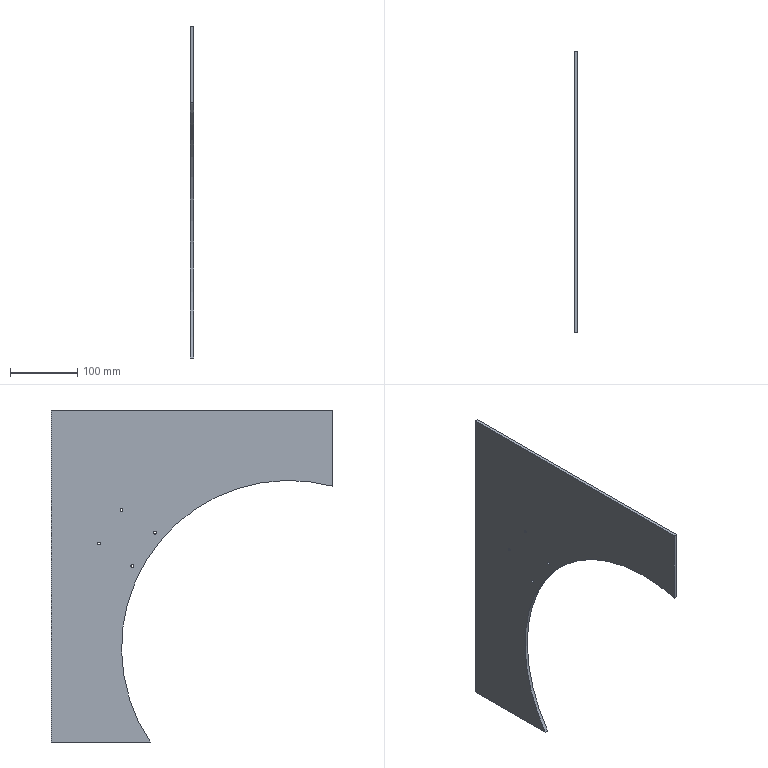Part | STEP file | 09-12 Outer base plate 1 | 1 solid | 15 faces | box 5 x 420 x 495 mm | volume 502595 mm3 | cylinder 9 | plane 6 | commonest cylinder face diameters 4.2 x8 500 x1
STEP:
#1=CARTESIAN_POINT('',(0.,0.,0.));
#2=DIRECTION('',(0.,0.,1.));
#3=DIRECTION('',(1.,0.,0.));
#4=AXIS2_PLACEMENT_3D('',#1,#2,#3);
#5=CARTESIAN_POINT('',(0.,348.664,-201.105));
#6=VERTEX_POINT('',#5);
#7=CARTESIAN_POINT('',(5.,348.664,-201.105));
#8=VERTEX_POINT('',#7);
#9=CARTESIAN_POINT('',(0.,348.664,-201.105));
#10=DIRECTION('',(1.,0.,0.));
#11=VECTOR('',#10,1.);
#12=LINE('',#9,#11);
#13=CARTESIAN_POINT('',(0.,348.664,-199.005));
#14=DIRECTION('',(1.,0.,0.));
#15=DIRECTION('',(0.,0.,-1.));
#16=AXIS2_PLACEMENT_3D('',#13,#14,#15);
#17=CYLINDRICAL_SURFACE('',#16,2.1);
#18=CARTESIAN_POINT('',(6.283,0.));
#19=DIRECTION('',(0.,1.));
#20=VECTOR('',#19,1.);
#21=LINE('',#18,#20);
#22=(GEOMETRIC_REPRESENTATION_CONTEXT(2)PARAMETRIC_REPRESENTATION_CONTEXT()REPRESENTATION_CONTEXT('',''));
#23=DEFINITIONAL_REPRESENTATION('',(#21),#22);
#24=PCURVE('',#17,#23);
#25=CARTESIAN_POINT('',(0.,348.664,-199.005));
#26=DIRECTION('',(1.,0.,0.));
#27=DIRECTION('',(0.,0.,-1.));
#28=AXIS2_PLACEMENT_3D('',#25,#26,#27);
#29=CYLINDRICAL_SURFACE('',#28,2.1);
#30=CARTESIAN_POINT('',(0.,0.));
#31=DIRECTION('',(0.,1.));
#32=VECTOR('',#31,1.);
#33=LINE('',#30,#32);
#34=(GEOMETRIC_REPRESENTATION_CONTEXT(2)PARAMETRIC_REPRESENTATION_CONTEXT()REPRESENTATION_CONTEXT('',''));
#35=DEFINITIONAL_REPRESENTATION('',(#33),#34);
#36=PCURVE('',#29,#35);
#37=SURFACE_CURVE('',#12,(#24,#36),.PCURVE_S1.);
#38=EDGE_CURVE('',#6,#8,#37,.T.);
#39=ORIENTED_EDGE('',*,*,#38,.T.);
#40=CARTESIAN_POINT('',(5.,348.664,-196.905));
#41=VERTEX_POINT('',#40);
#42=CARTESIAN_POINT('',(5.,348.664,-199.005));
#43=DIRECTION('',(1.,0.,0.));
#44=DIRECTION('',(0.,0.,-1.));
#45=AXIS2_PLACEMENT_3D('',#42,#43,#44);
#46=CIRCLE('',#45,2.1);
#47=CARTESIAN_POINT('',(0.,5.));
#48=DIRECTION('',(1.,0.));
#49=VECTOR('',#48,1.);
#50=LINE('',#47,#49);
#51=(GEOMETRIC_REPRESENTATION_CONTEXT(2)PARAMETRIC_REPRESENTATION_CONTEXT()REPRESENTATION_CONTEXT('',''));
#52=DEFINITIONAL_REPRESENTATION('',(#50),#51);
#53=PCURVE('',#17,#52);
#54=CARTESIAN_POINT('',(5.,0.,0.));
#55=DIRECTION('',(1.,0.,0.));
#56=DIRECTION('',(0.,0.,-1.));
#57=AXIS2_PLACEMENT_3D('',#54,#55,#56);
#58=PLANE('',#57);
#59=CARTESIAN_POINT('',(199.005,348.664));
#60=DIRECTION('',(1.,0.));
#61=AXIS2_PLACEMENT_2D('',#59,#60);
#62=CIRCLE('',#61,2.1);
#63=(GEOMETRIC_REPRESENTATION_CONTEXT(2)PARAMETRIC_REPRESENTATION_CONTEXT()REPRESENTATION_CONTEXT('',''));
#64=DEFINITIONAL_REPRESENTATION('',(#62),#63);
#65=PCURVE('',#58,#64);
#66=SURFACE_CURVE('',#46,(#53,#65),.PCURVE_S1.);
#67=EDGE_CURVE('',#41,#8,#66,.T.);
#68=ORIENTED_EDGE('',*,*,#67,.F.);
#69=CARTESIAN_POINT('',(0.,348.664,-196.905));
#70=VERTEX_POINT('',#69);
#71=CARTESIAN_POINT('',(0.,348.664,-196.905));
#72=DIRECTION('',(1.,0.,0.));
#73=VECTOR('',#72,1.);
#74=LINE('',#71,#73);
#75=CARTESIAN_POINT('',(3.142,0.));
#76=DIRECTION('',(0.,1.));
#77=VECTOR('',#76,1.);
#78=LINE('',#75,#77);
#79=(GEOMETRIC_REPRESENTATION_CONTEXT(2)PARAMETRIC_REPRESENTATION_CONTEXT()REPRESENTATION_CONTEXT('',''));
#80=DEFINITIONAL_REPRESENTATION('',(#78),#79);
#81=PCURVE('',#17,#80);
#82=CARTESIAN_POINT('',(3.142,0.));
#83=DIRECTION('',(0.,1.));
#84=VECTOR('',#83,1.);
#85=LINE('',#82,#84);
#86=(GEOMETRIC_REPRESENTATION_CONTEXT(2)PARAMETRIC_REPRESENTATION_CONTEXT()REPRESENTATION_CONTEXT('',''));
#87=DEFINITIONAL_REPRESENTATION('',(#85),#86);
#88=PCURVE('',#29,#87);
#89=SURFACE_CURVE('',#74,(#81,#88),.PCURVE_S1.);
#90=EDGE_CURVE('',#70,#41,#89,.T.);
#91=ORIENTED_EDGE('',*,*,#90,.F.);
#92=CARTESIAN_POINT('',(0.,348.664,-199.005));
#93=DIRECTION('',(-1.,0.,0.));
#94=DIRECTION('',(0.,0.,-1.));
#95=AXIS2_PLACEMENT_3D('',#92,#93,#94);
#96=CIRCLE('',#95,2.1);
#97=CARTESIAN_POINT('',(6.283,0.));
#98=DIRECTION('',(-1.,0.));
#99=VECTOR('',#98,1.);
#100=LINE('',#97,#99);
#101=(GEOMETRIC_REPRESENTATION_CONTEXT(2)PARAMETRIC_REPRESENTATION_CONTEXT()REPRESENTATION_CONTEXT('',''));
#102=DEFINITIONAL_REPRESENTATION('',(#100),#101);
#103=PCURVE('',#17,#102);
#104=CARTESIAN_POINT('',(0.,0.,0.));
#105=DIRECTION('',(1.,0.,0.));
#106=DIRECTION('',(0.,0.,-1.));
#107=AXIS2_PLACEMENT_3D('',#104,#105,#106);
#108=PLANE('',#107);
#109=CARTESIAN_POINT('',(201.105,348.664));
#110=CARTESIAN_POINT('',(201.105,345.027));
#111=CARTESIAN_POINT('',(197.955,346.846));
#112=CARTESIAN_POINT('',(194.805,348.664));
#113=CARTESIAN_POINT('',(197.955,350.483));
#114=CARTESIAN_POINT('',(201.105,352.302));
#115=CARTESIAN_POINT('',(201.105,348.664));
#116=(BOUNDED_CURVE()B_SPLINE_CURVE(2,(#109,#110,#111,#112,#113,#114,#115),.UNSPECIFIED.,.T.,.F.)B_SPLINE_CURVE_WITH_KNOTS((1,2,2,2,2,1),(-2.094,0.,2.094,4.189,6.283,8.378),.UNSPECIFIED.)CURVE()GEOMETRIC_REPRESENTATION_ITEM()RATIONAL_B_SPLINE_CURVE((1.,0.5,1.,0.5,1.,0.5,1.))REPRESENTATION_ITEM(''));
#117=(GEOMETRIC_REPRESENTATION_CONTEXT(2)PARAMETRIC_REPRESENTATION_CONTEXT()REPRESENTATION_CONTEXT('',''));
#118=DEFINITIONAL_REPRESENTATION('',(#116),#117);
#119=PCURVE('',#108,#118);
#120=SURFACE_CURVE('',#96,(#103,#119),.PCURVE_S1.);
#121=EDGE_CURVE('',#6,#70,#120,.T.);
#122=ORIENTED_EDGE('',*,*,#121,.F.);
#123=EDGE_LOOP('',(#39,#68,#91,#122));
#124=FACE_BOUND('',#123,.F.);
#125=ADVANCED_FACE('',(#124),#17,.F.);
#126=CARTESIAN_POINT('',(0.,265.336,-185.095));
#127=VERTEX_POINT('',#126);
#128=CARTESIAN_POINT('',(5.,265.336,-185.095));
#129=VERTEX_POINT('',#128);
#130=CARTESIAN_POINT('',(0.,265.336,-185.095));
#131=DIRECTION('',(1.,0.,0.));
#132=VECTOR('',#131,1.);
#133=LINE('',#130,#132);
#134=CARTESIAN_POINT('',(0.,265.336,-182.995));
#135=DIRECTION('',(1.,0.,0.));
#136=DIRECTION('',(0.,0.,-1.));
#137=AXIS2_PLACEMENT_3D('',#134,#135,#136);
#138=CYLINDRICAL_SURFACE('',#137,2.1);
#139=CARTESIAN_POINT('',(6.283,0.));
#140=DIRECTION('',(0.,1.));
#141=VECTOR('',#140,1.);
#142=LINE('',#139,#141);
#143=(GEOMETRIC_REPRESENTATION_CONTEXT(2)PARAMETRIC_REPRESENTATION_CONTEXT()REPRESENTATION_CONTEXT('',''));
#144=DEFINITIONAL_REPRESENTATION('',(#142),#143);
#145=PCURVE('',#138,#144);
#146=CARTESIAN_POINT('',(0.,265.336,-182.995));
#147=DIRECTION('',(1.,0.,0.));
#148=DIRECTION('',(0.,0.,-1.));
#149=AXIS2_PLACEMENT_3D('',#146,#147,#148);
#150=CYLINDRICAL_SURFACE('',#149,2.1);
#151=CARTESIAN_POINT('',(0.,0.));
#152=DIRECTION('',(0.,1.));
#153=VECTOR('',#152,1.);
#154=LINE('',#151,#153);
#155=(GEOMETRIC_REPRESENTATION_CONTEXT(2)PARAMETRIC_REPRESENTATION_CONTEXT()REPRESENTATION_CONTEXT('',''));
#156=DEFINITIONAL_REPRESENTATION('',(#154),#155);
#157=PCURVE('',#150,#156);
#158=SURFACE_CURVE('',#133,(#145,#157),.PCURVE_S1.);
#159=EDGE_CURVE('',#127,#129,#158,.T.);
#160=ORIENTED_EDGE('',*,*,#159,.T.);
#161=CARTESIAN_POINT('',(5.,265.336,-180.895));
#162=VERTEX_POINT('',#161);
#163=CARTESIAN_POINT('',(5.,265.336,-182.995));
#164=DIRECTION('',(-1.,0.,0.));
#165=DIRECTION('',(0.,0.,-1.));
#166=AXIS2_PLACEMENT_3D('',#163,#164,#165);
#167=CIRCLE('',#166,2.1);
#168=CARTESIAN_POINT('',(6.283,5.));
#169=DIRECTION('',(-1.,0.));
#170=VECTOR('',#169,1.);
#171=LINE('',#168,#170);
#172=(GEOMETRIC_REPRESENTATION_CONTEXT(2)PARAMETRIC_REPRESENTATION_CONTEXT()REPRESENTATION_CONTEXT('',''));
#173=DEFINITIONAL_REPRESENTATION('',(#171),#172);
#174=PCURVE('',#138,#173);
#175=CARTESIAN_POINT('',(185.095,265.336));
#176=CARTESIAN_POINT('',(185.095,261.698));
#177=CARTESIAN_POINT('',(181.945,263.517));
#178=CARTESIAN_POINT('',(178.795,265.336));
#179=CARTESIAN_POINT('',(181.945,267.154));
#180=CARTESIAN_POINT('',(185.095,268.973));
#181=CARTESIAN_POINT('',(185.095,265.336));
#182=(BOUNDED_CURVE()B_SPLINE_CURVE(2,(#175,#176,#177,#178,#179,#180,#181),.UNSPECIFIED.,.T.,.F.)B_SPLINE_CURVE_WITH_KNOTS((1,2,2,2,2,1),(-2.094,0.,2.094,4.189,6.283,8.378),.UNSPECIFIED.)CURVE()GEOMETRIC_REPRESENTATION_ITEM()RATIONAL_B_SPLINE_CURVE((1.,0.5,1.,0.5,1.,0.5,1.))REPRESENTATION_ITEM(''));
#183=(GEOMETRIC_REPRESENTATION_CONTEXT(2)PARAMETRIC_REPRESENTATION_CONTEXT()REPRESENTATION_CONTEXT('',''));
#184=DEFINITIONAL_REPRESENTATION('',(#182),#183);
#185=PCURVE('',#58,#184);
#186=SURFACE_CURVE('',#167,(#174,#185),.PCURVE_S1.);
#187=EDGE_CURVE('',#129,#162,#186,.T.);
#188=ORIENTED_EDGE('',*,*,#187,.T.);
#189=CARTESIAN_POINT('',(0.,265.336,-180.895));
#190=VERTEX_POINT('',#189);
#191=CARTESIAN_POINT('',(0.,265.336,-180.895));
#192=DIRECTION('',(1.,0.,0.));
#193=VECTOR('',#192,1.);
#194=LINE('',#191,#193);
#195=CARTESIAN_POINT('',(3.142,0.));
#196=DIRECTION('',(0.,1.));
#197=VECTOR('',#196,1.);
#198=LINE('',#195,#197);
#199=(GEOMETRIC_REPRESENTATION_CONTEXT(2)PARAMETRIC_REPRESENTATION_CONTEXT()REPRESENTATION_CONTEXT('',''));
#200=DEFINITIONAL_REPRESENTATION('',(#198),#199);
#201=PCURVE('',#138,#200);
#202=CARTESIAN_POINT('',(3.142,0.));
#203=DIRECTION('',(0.,1.));
#204=VECTOR('',#203,1.);
#205=LINE('',#202,#204);
#206=(GEOMETRIC_REPRESENTATION_CONTEXT(2)PARAMETRIC_REPRESENTATION_CONTEXT()REPRESENTATION_CONTEXT('',''));
#207=DEFINITIONAL_REPRESENTATION('',(#205),#206);
#208=PCURVE('',#150,#207);
#209=SURFACE_CURVE('',#194,(#201,#208),.PCURVE_S1.);
#210=EDGE_CURVE('',#190,#162,#209,.T.);
#211=ORIENTED_EDGE('',*,*,#210,.F.);
#212=CARTESIAN_POINT('',(0.,265.336,-182.995));
#213=DIRECTION('',(-1.,0.,0.));
#214=DIRECTION('',(0.,0.,-1.));
#215=AXIS2_PLACEMENT_3D('',#212,#213,#214);
#216=CIRCLE('',#215,2.1);
#217=CARTESIAN_POINT('',(6.283,0.));
#218=DIRECTION('',(-1.,0.));
#219=VECTOR('',#218,1.);
#220=LINE('',#217,#219);
#221=(GEOMETRIC_REPRESENTATION_CONTEXT(2)PARAMETRIC_REPRESENTATION_CONTEXT()REPRESENTATION_CONTEXT('',''));
#222=DEFINITIONAL_REPRESENTATION('',(#220),#221);
#223=PCURVE('',#138,#222);
#224=CARTESIAN_POINT('',(185.095,265.336));
#225=CARTESIAN_POINT('',(185.095,261.698));
#226=CARTESIAN_POINT('',(181.945,263.517));
#227=CARTESIAN_POINT('',(178.795,265.336));
#228=CARTESIAN_POINT('',(181.945,267.154));
#229=CARTESIAN_POINT('',(185.095,268.973));
#230=CARTESIAN_POINT('',(185.095,265.336));
#231=(BOUNDED_CURVE()B_SPLINE_CURVE(2,(#224,#225,#226,#227,#228,#229,#230),.UNSPECIFIED.,.T.,.F.)B_SPLINE_CURVE_WITH_KNOTS((1,2,2,2,2,1),(-2.094,0.,2.094,4.189,6.283,8.378),.UNSPECIFIED.)CURVE()GEOMETRIC_REPRESENTATION_ITEM()RATIONAL_B_SPLINE_CURVE((1.,0.5,1.,0.5,1.,0.5,1.))REPRESENTATION_ITEM(''));
#232=(GEOMETRIC_REPRESENTATION_CONTEXT(2)PARAMETRIC_REPRESENTATION_CONTEXT()REPRESENTATION_CONTEXT('',''));
#233=DEFINITIONAL_REPRESENTATION('',(#231),#232);
#234=PCURVE('',#108,#233);
#235=SURFACE_CURVE('',#216,(#223,#234),.PCURVE_S1.);
#236=EDGE_CURVE('',#127,#190,#235,.T.);
#237=ORIENTED_EDGE('',*,*,#236,.F.);
#238=EDGE_LOOP('',(#160,#188,#211,#237));
#239=FACE_BOUND('',#238,.F.);
#240=ADVANCED_FACE('',(#239),#138,.F.);
#241=CARTESIAN_POINT('',(0.,315.005,-151.436));
#242=VERTEX_POINT('',#241);
#243=CARTESIAN_POINT('',(5.,315.005,-151.436));
#244=VERTEX_POINT('',#243);
#245=CARTESIAN_POINT('',(0.,315.005,-151.436));
#246=DIRECTION('',(1.,0.,0.));
#247=VECTOR('',#246,1.);
#248=LINE('',#245,#247);
#249=CARTESIAN_POINT('',(0.,315.005,-149.336));
#250=DIRECTION('',(1.,0.,0.));
#251=DIRECTION('',(0.,0.,-1.));
#252=AXIS2_PLACEMENT_3D('',#249,#250,#251);
#253=CYLINDRICAL_SURFACE('',#252,2.1);
#254=CARTESIAN_POINT('',(6.283,0.));
#255=DIRECTION('',(0.,1.));
#256=VECTOR('',#255,1.);
#257=LINE('',#254,#256);
#258=(GEOMETRIC_REPRESENTATION_CONTEXT(2)PARAMETRIC_REPRESENTATION_CONTEXT()REPRESENTATION_CONTEXT('',''));
#259=DEFINITIONAL_REPRESENTATION('',(#257),#258);
#260=PCURVE('',#253,#259);
#261=CARTESIAN_POINT('',(0.,315.005,-149.336));
#262=DIRECTION('',(1.,0.,0.));
#263=DIRECTION('',(0.,0.,-1.));
#264=AXIS2_PLACEMENT_3D('',#261,#262,#263);
#265=CYLINDRICAL_SURFACE('',#264,2.1);
#266=CARTESIAN_POINT('',(0.,0.));
#267=DIRECTION('',(0.,1.));
#268=VECTOR('',#267,1.);
#269=LINE('',#266,#268);
#270=(GEOMETRIC_REPRESENTATION_CONTEXT(2)PARAMETRIC_REPRESENTATION_CONTEXT()REPRESENTATION_CONTEXT('',''));
#271=DEFINITIONAL_REPRESENTATION('',(#269),#270);
#272=PCURVE('',#265,#271);
#273=SURFACE_CURVE('',#248,(#260,#272),.PCURVE_S1.);
#274=EDGE_CURVE('',#242,#244,#273,.T.);
#275=ORIENTED_EDGE('',*,*,#274,.T.);
#276=CARTESIAN_POINT('',(5.,315.005,-147.236));
#277=VERTEX_POINT('',#276);
#278=CARTESIAN_POINT('',(5.,315.005,-149.336));
#279=DIRECTION('',(-1.,0.,0.));
#280=DIRECTION('',(0.,0.,-1.));
#281=AXIS2_PLACEMENT_3D('',#278,#279,#280);
#282=CIRCLE('',#281,2.1);
#283=CARTESIAN_POINT('',(6.283,5.));
#284=DIRECTION('',(-1.,0.));
#285=VECTOR('',#284,1.);
#286=LINE('',#283,#285);
#287=(GEOMETRIC_REPRESENTATION_CONTEXT(2)PARAMETRIC_REPRESENTATION_CONTEXT()REPRESENTATION_CONTEXT('',''));
#288=DEFINITIONAL_REPRESENTATION('',(#286),#287);
#289=PCURVE('',#253,#288);
#290=CARTESIAN_POINT('',(151.436,315.005));
#291=CARTESIAN_POINT('',(151.436,311.367));
#292=CARTESIAN_POINT('',(148.286,313.186));
#293=CARTESIAN_POINT('',(145.136,315.005));
#294=CARTESIAN_POINT('',(148.286,316.823));
#295=CARTESIAN_POINT('',(151.436,318.642));
#296=CARTESIAN_POINT('',(151.436,315.005));
#297=(BOUNDED_CURVE()B_SPLINE_CURVE(2,(#290,#291,#292,#293,#294,#295,#296),.UNSPECIFIED.,.T.,.F.)B_SPLINE_CURVE_WITH_KNOTS((1,2,2,2,2,1),(-2.094,0.,2.094,4.189,6.283,8.378),.UNSPECIFIED.)CURVE()GEOMETRIC_REPRESENTATION_ITEM()RATIONAL_B_SPLINE_CURVE((1.,0.5,1.,0.5,1.,0.5,1.))REPRESENTATION_ITEM(''));
#298=(GEOMETRIC_REPRESENTATION_CONTEXT(2)PARAMETRIC_REPRESENTATION_CONTEXT()REPRESENTATION_CONTEXT('',''));
#299=DEFINITIONAL_REPRESENTATION('',(#297),#298);
#300=PCURVE('',#58,#299);
#301=SURFACE_CURVE('',#282,(#289,#300),.PCURVE_S1.);
#302=EDGE_CURVE('',#244,#277,#301,.T.);
#303=ORIENTED_EDGE('',*,*,#302,.T.);
#304=CARTESIAN_POINT('',(0.,315.005,-147.236));
#305=VERTEX_POINT('',#304);
#306=CARTESIAN_POINT('',(0.,315.005,-147.236));
#307=DIRECTION('',(1.,0.,0.));
#308=VECTOR('',#307,1.);
#309=LINE('',#306,#308);
#310=CARTESIAN_POINT('',(3.142,0.));
#311=DIRECTION('',(0.,1.));
#312=VECTOR('',#311,1.);
#313=LINE('',#310,#312);
#314=(GEOMETRIC_REPRESENTATION_CONTEXT(2)PARAMETRIC_REPRESENTATION_CONTEXT()REPRESENTATION_CONTEXT('',''));
#315=DEFINITIONAL_REPRESENTATION('',(#313),#314);
#316=PCURVE('',#253,#315);
#317=CARTESIAN_POINT('',(3.142,0.));
#318=DIRECTION('',(0.,1.));
#319=VECTOR('',#318,1.);
#320=LINE('',#317,#319);
#321=(GEOMETRIC_REPRESENTATION_CONTEXT(2)PARAMETRIC_REPRESENTATION_CONTEXT()REPRESENTATION_CONTEXT('',''));
#322=DEFINITIONAL_REPRESENTATION('',(#320),#321);
#323=PCURVE('',#265,#322);
#324=SURFACE_CURVE('',#309,(#316,#323),.PCURVE_S1.);
#325=EDGE_CURVE('',#305,#277,#324,.T.);
#326=ORIENTED_EDGE('',*,*,#325,.F.);
#327=CARTESIAN_POINT('',(0.,315.005,-149.336));
#328=DIRECTION('',(-1.,0.,0.));
#329=DIRECTION('',(0.,0.,-1.));
#330=AXIS2_PLACEMENT_3D('',#327,#328,#329);
#331=CIRCLE('',#330,2.1);
#332=CARTESIAN_POINT('',(6.283,0.));
#333=DIRECTION('',(-1.,0.));
#334=VECTOR('',#333,1.);
#335=LINE('',#332,#334);
#336=(GEOMETRIC_REPRESENTATION_CONTEXT(2)PARAMETRIC_REPRESENTATION_CONTEXT()REPRESENTATION_CONTEXT('',''));
#337=DEFINITIONAL_REPRESENTATION('',(#335),#336);
#338=PCURVE('',#253,#337);
#339=CARTESIAN_POINT('',(151.436,315.005));
#340=CARTESIAN_POINT('',(151.436,311.367));
#341=CARTESIAN_POINT('',(148.286,313.186));
#342=CARTESIAN_POINT('',(145.136,315.005));
#343=CARTESIAN_POINT('',(148.286,316.823));
#344=CARTESIAN_POINT('',(151.436,318.642));
#345=CARTESIAN_POINT('',(151.436,315.005));
#346=(BOUNDED_CURVE()B_SPLINE_CURVE(2,(#339,#340,#341,#342,#343,#344,#345),.UNSPECIFIED.,.T.,.F.)B_SPLINE_CURVE_WITH_KNOTS((1,2,2,2,2,1),(-2.094,0.,2.094,4.189,6.283,8.378),.UNSPECIFIED.)CURVE()GEOMETRIC_REPRESENTATION_ITEM()RATIONAL_B_SPLINE_CURVE((1.,0.5,1.,0.5,1.,0.5,1.))REPRESENTATION_ITEM(''));
#347=(GEOMETRIC_REPRESENTATION_CONTEXT(2)PARAMETRIC_REPRESENTATION_CONTEXT()REPRESENTATION_CONTEXT('',''));
#348=DEFINITIONAL_REPRESENTATION('',(#346),#347);
#349=PCURVE('',#108,#348);
#350=SURFACE_CURVE('',#331,(#338,#349),.PCURVE_S1.);
#351=EDGE_CURVE('',#242,#305,#350,.T.);
#352=ORIENTED_EDGE('',*,*,#351,.F.);
#353=EDGE_LOOP('',(#275,#303,#326,#352));
#354=FACE_BOUND('',#353,.F.);
#355=ADVANCED_FACE('',(#354),#253,.F.);
#356=CARTESIAN_POINT('',(0.,298.995,-234.764));
#357=VERTEX_POINT('',#356);
#358=CARTESIAN_POINT('',(5.,298.995,-234.764));
#359=VERTEX_POINT('',#358);
#360=CARTESIAN_POINT('',(0.,298.995,-234.764));
#361=DIRECTION('',(1.,0.,0.));
#362=VECTOR('',#361,1.);
#363=LINE('',#360,#362);
#364=CARTESIAN_POINT('',(0.,298.995,-232.664));
#365=DIRECTION('',(1.,0.,0.));
#366=DIRECTION('',(0.,0.,-1.));
#367=AXIS2_PLACEMENT_3D('',#364,#365,#366);
#368=CYLINDRICAL_SURFACE('',#367,2.1);
#369=CARTESIAN_POINT('',(6.283,0.));
#370=DIRECTION('',(0.,1.));
#371=VECTOR('',#370,1.);
#372=LINE('',#369,#371);
#373=(GEOMETRIC_REPRESENTATION_CONTEXT(2)PARAMETRIC_REPRESENTATION_CONTEXT()REPRESENTATION_CONTEXT('',''));
#374=DEFINITIONAL_REPRESENTATION('',(#372),#373);
#375=PCURVE('',#368,#374);
#376=CARTESIAN_POINT('',(0.,298.995,-232.664));
#377=DIRECTION('',(1.,0.,0.));
#378=DIRECTION('',(0.,0.,-1.));
#379=AXIS2_PLACEMENT_3D('',#376,#377,#378);
#380=CYLINDRICAL_SURFACE('',#379,2.1);
#381=CARTESIAN_POINT('',(0.,0.));
#382=DIRECTION('',(0.,1.));
#383=VECTOR('',#382,1.);
#384=LINE('',#381,#383);
#385=(GEOMETRIC_REPRESENTATION_CONTEXT(2)PARAMETRIC_REPRESENTATION_CONTEXT()REPRESENTATION_CONTEXT('',''));
#386=DEFINITIONAL_REPRESENTATION('',(#384),#385);
#387=PCURVE('',#380,#386);
#388=SURFACE_CURVE('',#363,(#375,#387),.PCURVE_S1.);
#389=EDGE_CURVE('',#357,#359,#388,.T.);
#390=ORIENTED_EDGE('',*,*,#389,.T.);
#391=CARTESIAN_POINT('',(5.,298.995,-230.564));
#392=VERTEX_POINT('',#391);
#393=CARTESIAN_POINT('',(5.,298.995,-232.664));
#394=DIRECTION('',(-1.,0.,0.));
#395=DIRECTION('',(0.,0.,-1.));
#396=AXIS2_PLACEMENT_3D('',#393,#394,#395);
#397=CIRCLE('',#396,2.1);
#398=CARTESIAN_POINT('',(6.283,5.));
#399=DIRECTION('',(-1.,0.));
#400=VECTOR('',#399,1.);
#401=LINE('',#398,#400);
#402=(GEOMETRIC_REPRESENTATION_CONTEXT(2)PARAMETRIC_REPRESENTATION_CONTEXT()REPRESENTATION_CONTEXT('',''));
#403=DEFINITIONAL_REPRESENTATION('',(#401),#402);
#404=PCURVE('',#368,#403);
#405=CARTESIAN_POINT('',(234.764,298.995));
#406=CARTESIAN_POINT('',(234.764,295.358));
#407=CARTESIAN_POINT('',(231.614,297.177));
#408=CARTESIAN_POINT('',(228.464,298.995));
#409=CARTESIAN_POINT('',(231.614,300.814));
#410=CARTESIAN_POINT('',(234.764,302.633));
#411=CARTESIAN_POINT('',(234.764,298.995));
#412=(BOUNDED_CURVE()B_SPLINE_CURVE(2,(#405,#406,#407,#408,#409,#410,#411),.UNSPECIFIED.,.T.,.F.)B_SPLINE_CURVE_WITH_KNOTS((1,2,2,2,2,1),(-2.094,0.,2.094,4.189,6.283,8.378),.UNSPECIFIED.)CURVE()GEOMETRIC_REPRESENTATION_ITEM()RATIONAL_B_SPLINE_CURVE((1.,0.5,1.,0.5,1.,0.5,1.))REPRESENTATION_ITEM(''));
#413=(GEOMETRIC_REPRESENTATION_CONTEXT(2)PARAMETRIC_REPRESENTATION_CONTEXT()REPRESENTATION_CONTEXT('',''));
#414=DEFINITIONAL_REPRESENTATION('',(#412),#413);
#415=PCURVE('',#58,#414);
#416=SURFACE_CURVE('',#397,(#404,#415),.PCURVE_S1.);
#417=EDGE_CURVE('',#359,#392,#416,.T.);
#418=ORIENTED_EDGE('',*,*,#417,.T.);
#419=CARTESIAN_POINT('',(0.,298.995,-230.564));
#420=VERTEX_POINT('',#419);
#421=CARTESIAN_POINT('',(0.,298.995,-230.564));
#422=DIRECTION('',(1.,0.,0.));
#423=VECTOR('',#422,1.);
#424=LINE('',#421,#423);
#425=CARTESIAN_POINT('',(3.142,0.));
#426=DIRECTION('',(0.,1.));
#427=VECTOR('',#426,1.);
#428=LINE('',#425,#427);
#429=(GEOMETRIC_REPRESENTATION_CONTEXT(2)PARAMETRIC_REPRESENTATION_CONTEXT()REPRESENTATION_CONTEXT('',''));
#430=DEFINITIONAL_REPRESENTATION('',(#428),#429);
#431=PCURVE('',#368,#430);
#432=CARTESIAN_POINT('',(3.142,0.));
#433=DIRECTION('',(0.,1.));
#434=VECTOR('',#433,1.);
#435=LINE('',#432,#434);
#436=(GEOMETRIC_REPRESENTATION_CONTEXT(2)PARAMETRIC_REPRESENTATION_CONTEXT()REPRESENTATION_CONTEXT('',''));
#437=DEFINITIONAL_REPRESENTATION('',(#435),#436);
#438=PCURVE('',#380,#437);
#439=SURFACE_CURVE('',#424,(#431,#438),.PCURVE_S1.);
#440=EDGE_CURVE('',#420,#392,#439,.T.);
#441=ORIENTED_EDGE('',*,*,#440,.F.);
#442=CARTESIAN_POINT('',(0.,298.995,-232.664));
#443=DIRECTION('',(-1.,0.,0.));
#444=DIRECTION('',(0.,0.,-1.));
#445=AXIS2_PLACEMENT_3D('',#442,#443,#444);
#446=CIRCLE('',#445,2.1);
#447=CARTESIAN_POINT('',(6.283,0.));
#448=DIRECTION('',(-1.,0.));
#449=VECTOR('',#448,1.);
#450=LINE('',#447,#449);
#451=(GEOMETRIC_REPRESENTATION_CONTEXT(2)PARAMETRIC_REPRESENTATION_CONTEXT()REPRESENTATION_CONTEXT('',''));
#452=DEFINITIONAL_REPRESENTATION('',(#450),#451);
#453=PCURVE('',#368,#452);
#454=CARTESIAN_POINT('',(234.764,298.995));
#455=CARTESIAN_POINT('',(234.764,295.358));
#456=CARTESIAN_POINT('',(231.614,297.177));
#457=CARTESIAN_POINT('',(228.464,298.995));
#458=CARTESIAN_POINT('',(231.614,300.814));
#459=CARTESIAN_POINT('',(234.764,302.633));
#460=CARTESIAN_POINT('',(234.764,298.995));
#461=(BOUNDED_CURVE()B_SPLINE_CURVE(2,(#454,#455,#456,#457,#458,#459,#460),.UNSPECIFIED.,.T.,.F.)B_SPLINE_CURVE_WITH_KNOTS((1,2,2,2,2,1),(-2.094,0.,2.094,4.189,6.283,8.378),.UNSPECIFIED.)CURVE()GEOMETRIC_REPRESENTATION_ITEM()RATIONAL_B_SPLINE_CURVE((1.,0.5,1.,0.5,1.,0.5,1.))REPRESENTATION_ITEM(''));
#462=(GEOMETRIC_REPRESENTATION_CONTEXT(2)PARAMETRIC_REPRESENTATION_CONTEXT()REPRESENTATION_CONTEXT('',''));
#463=DEFINITIONAL_REPRESENTATION('',(#461),#462);
#464=PCURVE('',#108,#463);
#465=SURFACE_CURVE('',#446,(#453,#464),.PCURVE_S1.);
#466=EDGE_CURVE('',#357,#420,#465,.T.);
#467=ORIENTED_EDGE('',*,*,#466,.F.);
#468=EDGE_LOOP('',(#390,#418,#441,#467));
#469=FACE_BOUND('',#468,.F.);
#470=ADVANCED_FACE('',(#469),#368,.F.);
#471=CARTESIAN_POINT('',(5.,348.664,-199.005));
#472=DIRECTION('',(1.,0.,0.));
#473=DIRECTION('',(0.,0.,-1.));
#474=AXIS2_PLACEMENT_3D('',#471,#472,#473);
#475=CIRCLE('',#474,2.1);
#476=CARTESIAN_POINT('',(0.,5.));
#477=DIRECTION('',(1.,0.));
#478=VECTOR('',#477,1.);
#479=LINE('',#476,#478);
#480=(GEOMETRIC_REPRESENTATION_CONTEXT(2)PARAMETRIC_REPRESENTATION_CONTEXT()REPRESENTATION_CONTEXT('',''));
#481=DEFINITIONAL_REPRESENTATION('',(#479),#480);
#482=PCURVE('',#29,#481);
#483=CARTESIAN_POINT('',(199.005,348.664));
#484=DIRECTION('',(1.,0.));
#485=AXIS2_PLACEMENT_2D('',#483,#484);
#486=CIRCLE('',#485,2.1);
#487=(GEOMETRIC_REPRESENTATION_CONTEXT(2)PARAMETRIC_REPRESENTATION_CONTEXT()REPRESENTATION_CONTEXT('',''));
#488=DEFINITIONAL_REPRESENTATION('',(#486),#487);
#489=PCURVE('',#58,#488);
#490=SURFACE_CURVE('',#475,(#482,#489),.PCURVE_S1.);
#491=EDGE_CURVE('',#8,#41,#490,.T.);
#492=ORIENTED_EDGE('',*,*,#491,.F.);
#493=ORIENTED_EDGE('',*,*,#38,.F.);
#494=CARTESIAN_POINT('',(0.,348.664,-199.005));
#495=DIRECTION('',(-1.,0.,0.));
#496=DIRECTION('',(0.,0.,-1.));
#497=AXIS2_PLACEMENT_3D('',#494,#495,#496);
#498=CIRCLE('',#497,2.1);
#499=CARTESIAN_POINT('',(6.283,0.));
#500=DIRECTION('',(-1.,0.));
#501=VECTOR('',#500,1.);
#502=LINE('',#499,#501);
#503=(GEOMETRIC_REPRESENTATION_CONTEXT(2)PARAMETRIC_REPRESENTATION_CONTEXT()REPRESENTATION_CONTEXT('',''));
#504=DEFINITIONAL_REPRESENTATION('',(#502),#503);
#505=PCURVE('',#29,#504);
#506=CARTESIAN_POINT('',(201.105,348.664));
#507=CARTESIAN_POINT('',(201.105,345.027));
#508=CARTESIAN_POINT('',(197.955,346.846));
#509=CARTESIAN_POINT('',(194.805,348.664));
#510=CARTESIAN_POINT('',(197.955,350.483));
#511=CARTESIAN_POINT('',(201.105,352.302));
#512=CARTESIAN_POINT('',(201.105,348.664));
#513=(BOUNDED_CURVE()B_SPLINE_CURVE(2,(#506,#507,#508,#509,#510,#511,#512),.UNSPECIFIED.,.T.,.F.)B_SPLINE_CURVE_WITH_KNOTS((1,2,2,2,2,1),(-2.094,0.,2.094,4.189,6.283,8.378),.UNSPECIFIED.)CURVE()GEOMETRIC_REPRESENTATION_ITEM()RATIONAL_B_SPLINE_CURVE((1.,0.5,1.,0.5,1.,0.5,1.))REPRESENTATION_ITEM(''));
#514=(GEOMETRIC_REPRESENTATION_CONTEXT(2)PARAMETRIC_REPRESENTATION_CONTEXT()REPRESENTATION_CONTEXT('',''));
#515=DEFINITIONAL_REPRESENTATION('',(#513),#514);
#516=PCURVE('',#108,#515);
#517=SURFACE_CURVE('',#498,(#505,#516),.PCURVE_S1.);
#518=EDGE_CURVE('',#70,#6,#517,.T.);
#519=ORIENTED_EDGE('',*,*,#518,.F.);
#520=ORIENTED_EDGE('',*,*,#90,.T.);
#521=EDGE_LOOP('',(#492,#493,#519,#520));
#522=FACE_BOUND('',#521,.F.);
#523=ADVANCED_FACE('',(#522),#29,.F.);
#524=ORIENTED_EDGE('',*,*,#187,.T.);
#525=CARTESIAN_POINT('',(5.,265.336,-182.995));
#526=DIRECTION('',(-1.,0.,0.));
#527=DIRECTION('',(0.,0.,-1.));
#528=AXIS2_PLACEMENT_3D('',#525,#526,#527);
#529=CIRCLE('',#528,2.1);
#530=CARTESIAN_POINT('',(185.095,265.336));
#531=CARTESIAN_POINT('',(185.095,261.698));
#532=CARTESIAN_POINT('',(181.945,263.517));
#533=CARTESIAN_POINT('',(178.795,265.336));
#534=CARTESIAN_POINT('',(181.945,267.154));
#535=CARTESIAN_POINT('',(185.095,268.973));
#536=CARTESIAN_POINT('',(185.095,265.336));
#537=(BOUNDED_CURVE()B_SPLINE_CURVE(2,(#530,#531,#532,#533,#534,#535,#536),.UNSPECIFIED.,.T.,.F.)B_SPLINE_CURVE_WITH_KNOTS((1,2,2,2,2,1),(-2.094,0.,2.094,4.189,6.283,8.378),.UNSPECIFIED.)CURVE()GEOMETRIC_REPRESENTATION_ITEM()RATIONAL_B_SPLINE_CURVE((1.,0.5,1.,0.5,1.,0.5,1.))REPRESENTATION_ITEM(''));
#538=(GEOMETRIC_REPRESENTATION_CONTEXT(2)PARAMETRIC_REPRESENTATION_CONTEXT()REPRESENTATION_CONTEXT('',''));
#539=DEFINITIONAL_REPRESENTATION('',(#537),#538);
#540=PCURVE('',#58,#539);
#541=CARTESIAN_POINT('',(6.283,5.));
#542=DIRECTION('',(-1.,0.));
#543=VECTOR('',#542,1.);
#544=LINE('',#541,#543);
#545=(GEOMETRIC_REPRESENTATION_CONTEXT(2)PARAMETRIC_REPRESENTATION_CONTEXT()REPRESENTATION_CONTEXT('',''));
#546=DEFINITIONAL_REPRESENTATION('',(#544),#545);
#547=PCURVE('',#150,#546);
#548=SURFACE_CURVE('',#529,(#540,#547),.PCURVE_S1.);
#549=EDGE_CURVE('',#162,#129,#548,.T.);
#550=ORIENTED_EDGE('',*,*,#549,.T.);
#551=EDGE_LOOP('',(#524,#550));
#552=FACE_BOUND('',#551,.T.);
#553=ORIENTED_EDGE('',*,*,#302,.T.);
#554=CARTESIAN_POINT('',(5.,315.005,-149.336));
#555=DIRECTION('',(-1.,0.,0.));
#556=DIRECTION('',(0.,0.,-1.));
#557=AXIS2_PLACEMENT_3D('',#554,#555,#556);
#558=CIRCLE('',#557,2.1);
#559=CARTESIAN_POINT('',(151.436,315.005));
#560=CARTESIAN_POINT('',(151.436,311.367));
#561=CARTESIAN_POINT('',(148.286,313.186));
#562=CARTESIAN_POINT('',(145.136,315.005));
#563=CARTESIAN_POINT('',(148.286,316.823));
#564=CARTESIAN_POINT('',(151.436,318.642));
#565=CARTESIAN_POINT('',(151.436,315.005));
#566=(BOUNDED_CURVE()B_SPLINE_CURVE(2,(#559,#560,#561,#562,#563,#564,#565),.UNSPECIFIED.,.T.,.F.)B_SPLINE_CURVE_WITH_KNOTS((1,2,2,2,2,1),(-2.094,0.,2.094,4.189,6.283,8.378),.UNSPECIFIED.)CURVE()GEOMETRIC_REPRESENTATION_ITEM()RATIONAL_B_SPLINE_CURVE((1.,0.5,1.,0.5,1.,0.5,1.))REPRESENTATION_ITEM(''));
#567=(GEOMETRIC_REPRESENTATION_CONTEXT(2)PARAMETRIC_REPRESENTATION_CONTEXT()REPRESENTATION_CONTEXT('',''));
#568=DEFINITIONAL_REPRESENTATION('',(#566),#567);
#569=PCURVE('',#58,#568);
#570=CARTESIAN_POINT('',(6.283,5.));
#571=DIRECTION('',(-1.,0.));
#572=VECTOR('',#571,1.);
#573=LINE('',#570,#572);
#574=(GEOMETRIC_REPRESENTATION_CONTEXT(2)PARAMETRIC_REPRESENTATION_CONTEXT()REPRESENTATION_CONTEXT('',''));
#575=DEFINITIONAL_REPRESENTATION('',(#573),#574);
#576=PCURVE('',#265,#575);
#577=SURFACE_CURVE('',#558,(#569,#576),.PCURVE_S1.);
#578=EDGE_CURVE('',#277,#244,#577,.T.);
#579=ORIENTED_EDGE('',*,*,#578,.T.);
#580=EDGE_LOOP('',(#553,#579));
#581=FACE_BOUND('',#580,.T.);
#582=ORIENTED_EDGE('',*,*,#417,.T.);
#583=CARTESIAN_POINT('',(5.,298.995,-232.664));
#584=DIRECTION('',(-1.,0.,0.));
#585=DIRECTION('',(0.,0.,-1.));
#586=AXIS2_PLACEMENT_3D('',#583,#584,#585);
#587=CIRCLE('',#586,2.1);
#588=CARTESIAN_POINT('',(234.764,298.995));
#589=CARTESIAN_POINT('',(234.764,295.358));
#590=CARTESIAN_POINT('',(231.614,297.177));
#591=CARTESIAN_POINT('',(228.464,298.995));
#592=CARTESIAN_POINT('',(231.614,300.814));
#593=CARTESIAN_POINT('',(234.764,302.633));
#594=CARTESIAN_POINT('',(234.764,298.995));
#595=(BOUNDED_CURVE()B_SPLINE_CURVE(2,(#588,#589,#590,#591,#592,#593,#594),.UNSPECIFIED.,.T.,.F.)B_SPLINE_CURVE_WITH_KNOTS((1,2,2,2,2,1),(-2.094,0.,2.094,4.189,6.283,8.378),.UNSPECIFIED.)CURVE()GEOMETRIC_REPRESENTATION_ITEM()RATIONAL_B_SPLINE_CURVE((1.,0.5,1.,0.5,1.,0.5,1.))REPRESENTATION_ITEM(''));
#596=(GEOMETRIC_REPRESENTATION_CONTEXT(2)PARAMETRIC_REPRESENTATION_CONTEXT()REPRESENTATION_CONTEXT('',''));
#597=DEFINITIONAL_REPRESENTATION('',(#595),#596);
#598=PCURVE('',#58,#597);
#599=CARTESIAN_POINT('',(6.283,5.));
#600=DIRECTION('',(-1.,0.));
#601=VECTOR('',#600,1.);
#602=LINE('',#599,#601);
#603=(GEOMETRIC_REPRESENTATION_CONTEXT(2)PARAMETRIC_REPRESENTATION_CONTEXT()REPRESENTATION_CONTEXT('',''));
#604=DEFINITIONAL_REPRESENTATION('',(#602),#603);
#605=PCURVE('',#380,#604);
#606=SURFACE_CURVE('',#587,(#598,#605),.PCURVE_S1.);
#607=EDGE_CURVE('',#392,#359,#606,.T.);
#608=ORIENTED_EDGE('',*,*,#607,.T.);
#609=EDGE_LOOP('',(#582,#608));
#610=FACE_BOUND('',#609,.T.);
#611=ORIENTED_EDGE('',*,*,#491,.F.);
#612=ORIENTED_EDGE('',*,*,#67,.F.);
#613=EDGE_LOOP('',(#611,#612));
#614=FACE_BOUND('',#613,.T.);
#615=CARTESIAN_POINT('',(5.,272.123,-495.));
#616=VERTEX_POINT('',#615);
#617=CARTESIAN_POINT('',(5.,420.,-495.));
#618=VERTEX_POINT('',#617);
#619=CARTESIAN_POINT('',(5.,210.,-495.));
#620=DIRECTION('',(0.,1.,0.));
#621=VECTOR('',#620,1.);
#622=LINE('',#619,#621);
#623=CARTESIAN_POINT('',(495.,210.));
#624=DIRECTION('',(0.,1.));
#625=VECTOR('',#624,1.);
#626=LINE('',#623,#625);
#627=(GEOMETRIC_REPRESENTATION_CONTEXT(2)PARAMETRIC_REPRESENTATION_CONTEXT()REPRESENTATION_CONTEXT('',''));
#628=DEFINITIONAL_REPRESENTATION('',(#626),#627);
#629=PCURVE('',#58,#628);
#630=CARTESIAN_POINT('',(0.,272.123,-495.));
#631=DIRECTION('',(0.,0.,1.));
#632=DIRECTION('',(1.,0.,0.));
#633=AXIS2_PLACEMENT_3D('',#630,#631,#632);
#634=PLANE('',#633);
#635=CARTESIAN_POINT('',(5.,-62.123));
#636=DIRECTION('',(0.,1.));
#637=VECTOR('',#636,1.);
#638=LINE('',#635,#637);
#639=(GEOMETRIC_REPRESENTATION_CONTEXT(2)PARAMETRIC_REPRESENTATION_CONTEXT()REPRESENTATION_CONTEXT('',''));
#640=DEFINITIONAL_REPRESENTATION('',(#638),#639);
#641=PCURVE('',#634,#640);
#642=SURFACE_CURVE('',#622,(#629,#641),.PCURVE_S1.);
#643=EDGE_CURVE('',#616,#618,#642,.T.);
#644=ORIENTED_EDGE('',*,*,#643,.T.);
#645=CARTESIAN_POINT('',(5.,420.,0.));
#646=VERTEX_POINT('',#645);
#647=CARTESIAN_POINT('',(5.,420.,-247.5));
#648=DIRECTION('',(0.,0.,1.));
#649=VECTOR('',#648,1.);
#650=LINE('',#647,#649);
#651=CARTESIAN_POINT('',(247.5,420.));
#652=DIRECTION('',(-1.,0.));
#653=VECTOR('',#652,1.);
#654=LINE('',#651,#653);
#655=(GEOMETRIC_REPRESENTATION_CONTEXT(2)PARAMETRIC_REPRESENTATION_CONTEXT()REPRESENTATION_CONTEXT('',''));
#656=DEFINITIONAL_REPRESENTATION('',(#654),#655);
#657=PCURVE('',#58,#656);
#658=CARTESIAN_POINT('',(0.,420.,0.));
#659=DIRECTION('',(0.,-1.,0.));
#660=DIRECTION('',(0.,0.,-1.));
#661=AXIS2_PLACEMENT_3D('',#658,#659,#660);
#662=PLANE('',#661);
#663=CARTESIAN_POINT('',(247.5,5.));
#664=DIRECTION('',(-1.,0.));
#665=VECTOR('',#664,1.);
#666=LINE('',#663,#665);
#667=(GEOMETRIC_REPRESENTATION_CONTEXT(2)PARAMETRIC_REPRESENTATION_CONTEXT()REPRESENTATION_CONTEXT('',''));
#668=DEFINITIONAL_REPRESENTATION('',(#666),#667);
#669=PCURVE('',#662,#668);
#670=SURFACE_CURVE('',#650,(#657,#669),.PCURVE_S1.);
#671=EDGE_CURVE('',#618,#646,#670,.T.);
#672=ORIENTED_EDGE('',*,*,#671,.T.);
#673=CARTESIAN_POINT('',(5.,0.,0.));
#674=VERTEX_POINT('',#673);
#675=CARTESIAN_POINT('',(5.,210.,0.));
#676=DIRECTION('',(0.,-1.,0.));
#677=VECTOR('',#676,1.);
#678=LINE('',#675,#677);
#679=CARTESIAN_POINT('',(0.,210.));
#680=DIRECTION('',(0.,-1.));
#681=VECTOR('',#680,1.);
#682=LINE('',#679,#681);
#683=(GEOMETRIC_REPRESENTATION_CONTEXT(2)PARAMETRIC_REPRESENTATION_CONTEXT()REPRESENTATION_CONTEXT('',''));
#684=DEFINITIONAL_REPRESENTATION('',(#682),#683);
#685=PCURVE('',#58,#684);
#686=CARTESIAN_POINT('',(5.,0.,0.));
#687=DIRECTION('',(0.,0.,-1.));
#688=DIRECTION('',(-1.,0.,0.));
#689=AXIS2_PLACEMENT_3D('',#686,#687,#688);
#690=PLANE('',#689);
#691=CARTESIAN_POINT('',(0.,210.));
#692=DIRECTION('',(0.,-1.));
#693=VECTOR('',#692,1.);
#694=LINE('',#691,#693);
#695=(GEOMETRIC_REPRESENTATION_CONTEXT(2)PARAMETRIC_REPRESENTATION_CONTEXT()REPRESENTATION_CONTEXT('',''));
#696=DEFINITIONAL_REPRESENTATION('',(#694),#695);
#697=PCURVE('',#690,#696);
#698=SURFACE_CURVE('',#678,(#685,#697),.PCURVE_S1.);
#699=EDGE_CURVE('',#646,#674,#698,.T.);
#700=ORIENTED_EDGE('',*,*,#699,.T.);
#701=CARTESIAN_POINT('',(5.,-0.000000033,-113.598));
#702=VERTEX_POINT('',#701);
#703=CARTESIAN_POINT('',(5.,0.,-247.5));
#704=DIRECTION('',(0.,0.,-1.));
#705=VECTOR('',#704,1.);
#706=LINE('',#703,#705);
#707=CARTESIAN_POINT('',(247.5,0.));
#708=DIRECTION('',(1.,0.));
#709=VECTOR('',#708,1.);
#710=LINE('',#707,#709);
#711=(GEOMETRIC_REPRESENTATION_CONTEXT(2)PARAMETRIC_REPRESENTATION_CONTEXT()REPRESENTATION_CONTEXT('',''));
#712=DEFINITIONAL_REPRESENTATION('',(#710),#711);
#713=PCURVE('',#58,#712);
#714=CARTESIAN_POINT('',(0.,0.,-113.598));
#715=DIRECTION('',(0.,1.,0.));
#716=DIRECTION('',(0.,0.,1.));
#717=AXIS2_PLACEMENT_3D('',#714,#715,#716);
#718=PLANE('',#717);
#719=CARTESIAN_POINT('',(-133.902,5.));
#720=DIRECTION('',(-1.,0.));
#721=VECTOR('',#720,1.);
#722=LINE('',#719,#721);
#723=(GEOMETRIC_REPRESENTATION_CONTEXT(2)PARAMETRIC_REPRESENTATION_CONTEXT()REPRESENTATION_CONTEXT('',''));
#724=DEFINITIONAL_REPRESENTATION('',(#722),#723);
#725=PCURVE('',#718,#724);
#726=SURFACE_CURVE('',#706,(#713,#725),.PCURVE_S1.);
#727=EDGE_CURVE('',#674,#702,#726,.T.);
#728=ORIENTED_EDGE('',*,*,#727,.T.);
#729=CARTESIAN_POINT('',(5.,65.,-355.));
#730=DIRECTION('',(-1.,0.,0.));
#731=DIRECTION('',(0.,-1.,0.));
#732=AXIS2_PLACEMENT_3D('',#729,#730,#731);
#733=CIRCLE('',#732,250.);
#734=CARTESIAN_POINT('',(355.,-185.));
#735=CARTESIAN_POINT('',(-78.013,-185.));
#736=CARTESIAN_POINT('',(138.494,190.));
#737=CARTESIAN_POINT('',(355.,565.));
#738=CARTESIAN_POINT('',(571.506,190.));
#739=CARTESIAN_POINT('',(788.013,-185.));
#740=CARTESIAN_POINT('',(355.,-185.));
#741=(BOUNDED_CURVE()B_SPLINE_CURVE(2,(#734,#735,#736,#737,#738,#739,#740),.UNSPECIFIED.,.T.,.F.)B_SPLINE_CURVE_WITH_KNOTS((1,2,2,2,2,1),(-2.094,0.,2.094,4.189,6.283,8.378),.UNSPECIFIED.)CURVE()GEOMETRIC_REPRESENTATION_ITEM()RATIONAL_B_SPLINE_CURVE((1.,0.5,1.,0.5,1.,0.5,1.))REPRESENTATION_ITEM(''));
#742=(GEOMETRIC_REPRESENTATION_CONTEXT(2)PARAMETRIC_REPRESENTATION_CONTEXT()REPRESENTATION_CONTEXT('',''));
#743=DEFINITIONAL_REPRESENTATION('',(#741),#742);
#744=PCURVE('',#58,#743);
#745=CARTESIAN_POINT('',(5.,65.,-355.));
#746=DIRECTION('',(-1.,0.,0.));
#747=DIRECTION('',(0.,-1.,0.));
#748=AXIS2_PLACEMENT_3D('',#745,#746,#747);
#749=CYLINDRICAL_SURFACE('',#748,250.);
#750=CARTESIAN_POINT('',(0.,0.));
#751=DIRECTION('',(1.,0.));
#752=VECTOR('',#751,1.);
#753=LINE('',#750,#752);
#754=(GEOMETRIC_REPRESENTATION_CONTEXT(2)PARAMETRIC_REPRESENTATION_CONTEXT()REPRESENTATION_CONTEXT('',''));
#755=DEFINITIONAL_REPRESENTATION('',(#753),#754);
#756=PCURVE('',#749,#755);
#757=SURFACE_CURVE('',#733,(#744,#756),.PCURVE_S1.);
#758=EDGE_CURVE('',#702,#616,#757,.T.);
#759=ORIENTED_EDGE('',*,*,#758,.T.);
#760=EDGE_LOOP('',(#644,#672,#700,#728,#759));
#761=FACE_BOUND('',#760,.T.);
#762=ADVANCED_FACE('',(#552,#581,#610,#614,#761),#58,.T.);
#763=ORIENTED_EDGE('',*,*,#236,.F.);
#764=CARTESIAN_POINT('',(0.,265.336,-182.995));
#765=DIRECTION('',(-1.,0.,0.));
#766=DIRECTION('',(0.,0.,-1.));
#767=AXIS2_PLACEMENT_3D('',#764,#765,#766);
#768=CIRCLE('',#767,2.1);
#769=CARTESIAN_POINT('',(185.095,265.336));
#770=CARTESIAN_POINT('',(185.095,261.698));
#771=CARTESIAN_POINT('',(181.945,263.517));
#772=CARTESIAN_POINT('',(178.795,265.336));
#773=CARTESIAN_POINT('',(181.945,267.154));
#774=CARTESIAN_POINT('',(185.095,268.973));
#775=CARTESIAN_POINT('',(185.095,265.336));
#776=(BOUNDED_CURVE()B_SPLINE_CURVE(2,(#769,#770,#771,#772,#773,#774,#775),.UNSPECIFIED.,.T.,.F.)B_SPLINE_CURVE_WITH_KNOTS((1,2,2,2,2,1),(-2.094,0.,2.094,4.189,6.283,8.378),.UNSPECIFIED.)CURVE()GEOMETRIC_REPRESENTATION_ITEM()RATIONAL_B_SPLINE_CURVE((1.,0.5,1.,0.5,1.,0.5,1.))REPRESENTATION_ITEM(''));
#777=(GEOMETRIC_REPRESENTATION_CONTEXT(2)PARAMETRIC_REPRESENTATION_CONTEXT()REPRESENTATION_CONTEXT('',''));
#778=DEFINITIONAL_REPRESENTATION('',(#776),#777);
#779=PCURVE('',#108,#778);
#780=CARTESIAN_POINT('',(6.283,0.));
#781=DIRECTION('',(-1.,0.));
#782=VECTOR('',#781,1.);
#783=LINE('',#780,#782);
#784=(GEOMETRIC_REPRESENTATION_CONTEXT(2)PARAMETRIC_REPRESENTATION_CONTEXT()REPRESENTATION_CONTEXT('',''));
#785=DEFINITIONAL_REPRESENTATION('',(#783),#784);
#786=PCURVE('',#150,#785);
#787=SURFACE_CURVE('',#768,(#779,#786),.PCURVE_S1.);
#788=EDGE_CURVE('',#190,#127,#787,.T.);
#789=ORIENTED_EDGE('',*,*,#788,.F.);
#790=EDGE_LOOP('',(#763,#789));
#791=FACE_BOUND('',#790,.T.);
#792=ORIENTED_EDGE('',*,*,#351,.F.);
#793=CARTESIAN_POINT('',(0.,315.005,-149.336));
#794=DIRECTION('',(-1.,0.,0.));
#795=DIRECTION('',(0.,0.,-1.));
#796=AXIS2_PLACEMENT_3D('',#793,#794,#795);
#797=CIRCLE('',#796,2.1);
#798=CARTESIAN_POINT('',(151.436,315.005));
#799=CARTESIAN_POINT('',(151.436,311.367));
#800=CARTESIAN_POINT('',(148.286,313.186));
#801=CARTESIAN_POINT('',(145.136,315.005));
#802=CARTESIAN_POINT('',(148.286,316.823));
#803=CARTESIAN_POINT('',(151.436,318.642));
#804=CARTESIAN_POINT('',(151.436,315.005));
#805=(BOUNDED_CURVE()B_SPLINE_CURVE(2,(#798,#799,#800,#801,#802,#803,#804),.UNSPECIFIED.,.T.,.F.)B_SPLINE_CURVE_WITH_KNOTS((1,2,2,2,2,1),(-2.094,0.,2.094,4.189,6.283,8.378),.UNSPECIFIED.)CURVE()GEOMETRIC_REPRESENTATION_ITEM()RATIONAL_B_SPLINE_CURVE((1.,0.5,1.,0.5,1.,0.5,1.))REPRESENTATION_ITEM(''));
#806=(GEOMETRIC_REPRESENTATION_CONTEXT(2)PARAMETRIC_REPRESENTATION_CONTEXT()REPRESENTATION_CONTEXT('',''));
#807=DEFINITIONAL_REPRESENTATION('',(#805),#806);
#808=PCURVE('',#108,#807);
#809=CARTESIAN_POINT('',(6.283,0.));
#810=DIRECTION('',(-1.,0.));
#811=VECTOR('',#810,1.);
#812=LINE('',#809,#811);
#813=(GEOMETRIC_REPRESENTATION_CONTEXT(2)PARAMETRIC_REPRESENTATION_CONTEXT()REPRESENTATION_CONTEXT('',''));
#814=DEFINITIONAL_REPRESENTATION('',(#812),#813);
#815=PCURVE('',#265,#814);
#816=SURFACE_CURVE('',#797,(#808,#815),.PCURVE_S1.);
#817=EDGE_CURVE('',#305,#242,#816,.T.);
#818=ORIENTED_EDGE('',*,*,#817,.F.);
#819=EDGE_LOOP('',(#792,#818));
#820=FACE_BOUND('',#819,.T.);
#821=ORIENTED_EDGE('',*,*,#466,.F.);
#822=CARTESIAN_POINT('',(0.,298.995,-232.664));
#823=DIRECTION('',(-1.,0.,0.));
#824=DIRECTION('',(0.,0.,-1.));
#825=AXIS2_PLACEMENT_3D('',#822,#823,#824);
#826=CIRCLE('',#825,2.1);
#827=CARTESIAN_POINT('',(234.764,298.995));
#828=CARTESIAN_POINT('',(234.764,295.358));
#829=CARTESIAN_POINT('',(231.614,297.177));
#830=CARTESIAN_POINT('',(228.464,298.995));
#831=CARTESIAN_POINT('',(231.614,300.814));
#832=CARTESIAN_POINT('',(234.764,302.633));
#833=CARTESIAN_POINT('',(234.764,298.995));
#834=(BOUNDED_CURVE()B_SPLINE_CURVE(2,(#827,#828,#829,#830,#831,#832,#833),.UNSPECIFIED.,.T.,.F.)B_SPLINE_CURVE_WITH_KNOTS((1,2,2,2,2,1),(-2.094,0.,2.094,4.189,6.283,8.378),.UNSPECIFIED.)CURVE()GEOMETRIC_REPRESENTATION_ITEM()RATIONAL_B_SPLINE_CURVE((1.,0.5,1.,0.5,1.,0.5,1.))REPRESENTATION_ITEM(''));
#835=(GEOMETRIC_REPRESENTATION_CONTEXT(2)PARAMETRIC_REPRESENTATION_CONTEXT()REPRESENTATION_CONTEXT('',''));
#836=DEFINITIONAL_REPRESENTATION('',(#834),#835);
#837=PCURVE('',#108,#836);
#838=CARTESIAN_POINT('',(6.283,0.));
#839=DIRECTION('',(-1.,0.));
#840=VECTOR('',#839,1.);
#841=LINE('',#838,#840);
#842=(GEOMETRIC_REPRESENTATION_CONTEXT(2)PARAMETRIC_REPRESENTATION_CONTEXT()REPRESENTATION_CONTEXT('',''));
#843=DEFINITIONAL_REPRESENTATION('',(#841),#842);
#844=PCURVE('',#380,#843);
#845=SURFACE_CURVE('',#826,(#837,#844),.PCURVE_S1.);
#846=EDGE_CURVE('',#420,#357,#845,.T.);
#847=ORIENTED_EDGE('',*,*,#846,.F.);
#848=EDGE_LOOP('',(#821,#847));
#849=FACE_BOUND('',#848,.T.);
#850=ORIENTED_EDGE('',*,*,#121,.F.);
#851=ORIENTED_EDGE('',*,*,#518,.F.);
#852=EDGE_LOOP('',(#850,#851));
#853=FACE_BOUND('',#852,.T.);
#854=CARTESIAN_POINT('',(0.,420.,-495.));
#855=VERTEX_POINT('',#854);
#856=CARTESIAN_POINT('',(0.,420.,0.));
#857=VERTEX_POINT('',#856);
#858=CARTESIAN_POINT('',(0.,420.,-247.5));
#859=DIRECTION('',(0.,0.,1.));
#860=VECTOR('',#859,1.);
#861=LINE('',#858,#860);
#862=CARTESIAN_POINT('',(247.5,420.));
#863=DIRECTION('',(-1.,0.));
#864=VECTOR('',#863,1.);
#865=LINE('',#862,#864);
#866=(GEOMETRIC_REPRESENTATION_CONTEXT(2)PARAMETRIC_REPRESENTATION_CONTEXT()REPRESENTATION_CONTEXT('',''));
#867=DEFINITIONAL_REPRESENTATION('',(#865),#866);
#868=PCURVE('',#108,#867);
#869=CARTESIAN_POINT('',(247.5,0.));
#870=DIRECTION('',(-1.,0.));
#871=VECTOR('',#870,1.);
#872=LINE('',#869,#871);
#873=(GEOMETRIC_REPRESENTATION_CONTEXT(2)PARAMETRIC_REPRESENTATION_CONTEXT()REPRESENTATION_CONTEXT('',''));
#874=DEFINITIONAL_REPRESENTATION('',(#872),#873);
#875=PCURVE('',#662,#874);
#876=SURFACE_CURVE('',#861,(#868,#875),.PCURVE_S1.);
#877=EDGE_CURVE('',#855,#857,#876,.T.);
#878=ORIENTED_EDGE('',*,*,#877,.F.);
#879=CARTESIAN_POINT('',(0.,272.123,-495.));
#880=VERTEX_POINT('',#879);
#881=CARTESIAN_POINT('',(0.,210.,-495.));
#882=DIRECTION('',(0.,1.,0.));
#883=VECTOR('',#882,1.);
#884=LINE('',#881,#883);
#885=CARTESIAN_POINT('',(495.,210.));
#886=DIRECTION('',(0.,1.));
#887=VECTOR('',#886,1.);
#888=LINE('',#885,#887);
#889=(GEOMETRIC_REPRESENTATION_CONTEXT(2)PARAMETRIC_REPRESENTATION_CONTEXT()REPRESENTATION_CONTEXT('',''));
#890=DEFINITIONAL_REPRESENTATION('',(#888),#889);
#891=PCURVE('',#108,#890);
#892=CARTESIAN_POINT('',(0.,-62.123));
#893=DIRECTION('',(0.,1.));
#894=VECTOR('',#893,1.);
#895=LINE('',#892,#894);
#896=(GEOMETRIC_REPRESENTATION_CONTEXT(2)PARAMETRIC_REPRESENTATION_CONTEXT()REPRESENTATION_CONTEXT('',''));
#897=DEFINITIONAL_REPRESENTATION('',(#895),#896);
#898=PCURVE('',#634,#897);
#899=SURFACE_CURVE('',#884,(#891,#898),.PCURVE_S1.);
#900=EDGE_CURVE('',#880,#855,#899,.T.);
#901=ORIENTED_EDGE('',*,*,#900,.F.);
#902=CARTESIAN_POINT('',(0.,-0.000000033,-113.598));
#903=VERTEX_POINT('',#902);
#904=CARTESIAN_POINT('',(0.,65.,-355.));
#905=DIRECTION('',(-1.,0.,0.));
#906=DIRECTION('',(0.,-1.,0.));
#907=AXIS2_PLACEMENT_3D('',#904,#905,#906);
#908=CIRCLE('',#907,250.);
#909=CARTESIAN_POINT('',(355.,-185.));
#910=CARTESIAN_POINT('',(-78.013,-185.));
#911=CARTESIAN_POINT('',(138.494,190.));
#912=CARTESIAN_POINT('',(355.,565.));
#913=CARTESIAN_POINT('',(571.506,190.));
#914=CARTESIAN_POINT('',(788.013,-185.));
#915=CARTESIAN_POINT('',(355.,-185.));
#916=(BOUNDED_CURVE()B_SPLINE_CURVE(2,(#909,#910,#911,#912,#913,#914,#915),.UNSPECIFIED.,.T.,.F.)B_SPLINE_CURVE_WITH_KNOTS((1,2,2,2,2,1),(-2.094,0.,2.094,4.189,6.283,8.378),.UNSPECIFIED.)CURVE()GEOMETRIC_REPRESENTATION_ITEM()RATIONAL_B_SPLINE_CURVE((1.,0.5,1.,0.5,1.,0.5,1.))REPRESENTATION_ITEM(''));
#917=(GEOMETRIC_REPRESENTATION_CONTEXT(2)PARAMETRIC_REPRESENTATION_CONTEXT()REPRESENTATION_CONTEXT('',''));
#918=DEFINITIONAL_REPRESENTATION('',(#916),#917);
#919=PCURVE('',#108,#918);
#920=CARTESIAN_POINT('',(0.,5.));
#921=DIRECTION('',(1.,0.));
#922=VECTOR('',#921,1.);
#923=LINE('',#920,#922);
#924=(GEOMETRIC_REPRESENTATION_CONTEXT(2)PARAMETRIC_REPRESENTATION_CONTEXT()REPRESENTATION_CONTEXT('',''));
#925=DEFINITIONAL_REPRESENTATION('',(#923),#924);
#926=PCURVE('',#749,#925);
#927=SURFACE_CURVE('',#908,(#919,#926),.PCURVE_S1.);
#928=EDGE_CURVE('',#903,#880,#927,.T.);
#929=ORIENTED_EDGE('',*,*,#928,.F.);
#930=CARTESIAN_POINT('',(0.,0.,0.));
#931=VERTEX_POINT('',#930);
#932=CARTESIAN_POINT('',(0.,0.,-247.5));
#933=DIRECTION('',(0.,0.,-1.));
#934=VECTOR('',#933,1.);
#935=LINE('',#932,#934);
#936=CARTESIAN_POINT('',(247.5,0.));
#937=DIRECTION('',(1.,0.));
#938=VECTOR('',#937,1.);
#939=LINE('',#936,#938);
#940=(GEOMETRIC_REPRESENTATION_CONTEXT(2)PARAMETRIC_REPRESENTATION_CONTEXT()REPRESENTATION_CONTEXT('',''));
#941=DEFINITIONAL_REPRESENTATION('',(#939),#940);
#942=PCURVE('',#108,#941);
#943=CARTESIAN_POINT('',(-133.902,0.));
#944=DIRECTION('',(-1.,0.));
#945=VECTOR('',#944,1.);
#946=LINE('',#943,#945);
#947=(GEOMETRIC_REPRESENTATION_CONTEXT(2)PARAMETRIC_REPRESENTATION_CONTEXT()REPRESENTATION_CONTEXT('',''));
#948=DEFINITIONAL_REPRESENTATION('',(#946),#947);
#949=PCURVE('',#718,#948);
#950=SURFACE_CURVE('',#935,(#942,#949),.PCURVE_S1.);
#951=EDGE_CURVE('',#931,#903,#950,.T.);
#952=ORIENTED_EDGE('',*,*,#951,.F.);
#953=CARTESIAN_POINT('',(0.,210.,0.));
#954=DIRECTION('',(0.,-1.,0.));
#955=VECTOR('',#954,1.);
#956=LINE('',#953,#955);
#957=CARTESIAN_POINT('',(0.,210.));
#958=DIRECTION('',(0.,-1.));
#959=VECTOR('',#958,1.);
#960=LINE('',#957,#959);
#961=(GEOMETRIC_REPRESENTATION_CONTEXT(2)PARAMETRIC_REPRESENTATION_CONTEXT()REPRESENTATION_CONTEXT('',''));
#962=DEFINITIONAL_REPRESENTATION('',(#960),#961);
#963=PCURVE('',#108,#962);
#964=CARTESIAN_POINT('',(5.,210.));
#965=DIRECTION('',(0.,-1.));
#966=VECTOR('',#965,1.);
#967=LINE('',#964,#966);
#968=(GEOMETRIC_REPRESENTATION_CONTEXT(2)PARAMETRIC_REPRESENTATION_CONTEXT()REPRESENTATION_CONTEXT('',''));
#969=DEFINITIONAL_REPRESENTATION('',(#967),#968);
#970=PCURVE('',#690,#969);
#971=SURFACE_CURVE('',#956,(#963,#970),.PCURVE_S1.);
#972=EDGE_CURVE('',#857,#931,#971,.T.);
#973=ORIENTED_EDGE('',*,*,#972,.F.);
#974=EDGE_LOOP('',(#878,#901,#929,#952,#973));
#975=FACE_BOUND('',#974,.T.);
#976=ADVANCED_FACE('',(#791,#820,#849,#853,#975),#108,.F.);
#977=ORIENTED_EDGE('',*,*,#549,.T.);
#978=ORIENTED_EDGE('',*,*,#159,.F.);
#979=ORIENTED_EDGE('',*,*,#788,.F.);
#980=ORIENTED_EDGE('',*,*,#210,.T.);
#981=EDGE_LOOP('',(#977,#978,#979,#980));
#982=FACE_BOUND('',#981,.F.);
#983=ADVANCED_FACE('',(#982),#150,.F.);
#984=ORIENTED_EDGE('',*,*,#578,.T.);
#985=ORIENTED_EDGE('',*,*,#274,.F.);
#986=ORIENTED_EDGE('',*,*,#817,.F.);
#987=ORIENTED_EDGE('',*,*,#325,.T.);
#988=EDGE_LOOP('',(#984,#985,#986,#987));
#989=FACE_BOUND('',#988,.F.);
#990=ADVANCED_FACE('',(#989),#265,.F.);
#991=ORIENTED_EDGE('',*,*,#607,.T.);
#992=ORIENTED_EDGE('',*,*,#389,.F.);
#993=ORIENTED_EDGE('',*,*,#846,.F.);
#994=ORIENTED_EDGE('',*,*,#440,.T.);
#995=EDGE_LOOP('',(#991,#992,#993,#994));
#996=FACE_BOUND('',#995,.F.);
#997=ADVANCED_FACE('',(#996),#380,.F.);
#998=CARTESIAN_POINT('',(2.5,420.,0.));
#999=DIRECTION('',(-1.,0.,0.));
#1000=VECTOR('',#999,1.);
#1001=LINE('',#998,#1000);
#1002=CARTESIAN_POINT('',(0.,2.5));
#1003=DIRECTION('',(0.,-1.));
#1004=VECTOR('',#1003,1.);
#1005=LINE('',#1002,#1004);
#1006=(GEOMETRIC_REPRESENTATION_CONTEXT(2)PARAMETRIC_REPRESENTATION_CONTEXT()REPRESENTATION_CONTEXT('',''));
#1007=DEFINITIONAL_REPRESENTATION('',(#1005),#1006);
#1008=PCURVE('',#662,#1007);
#1009=CARTESIAN_POINT('',(2.5,420.));
#1010=DIRECTION('',(1.,0.));
#1011=VECTOR('',#1010,1.);
#1012=LINE('',#1009,#1011);
#1013=(GEOMETRIC_REPRESENTATION_CONTEXT(2)PARAMETRIC_REPRESENTATION_CONTEXT()REPRESENTATION_CONTEXT('',''));
#1014=DEFINITIONAL_REPRESENTATION('',(#1012),#1013);
#1015=PCURVE('',#690,#1014);
#1016=SURFACE_CURVE('',#1001,(#1008,#1015),.PCURVE_S1.);
#1017=EDGE_CURVE('',#646,#857,#1016,.T.);
#1018=ORIENTED_EDGE('',*,*,#1017,.F.);
#1019=ORIENTED_EDGE('',*,*,#671,.F.);
#1020=CARTESIAN_POINT('',(2.5,420.,-495.));
#1021=DIRECTION('',(1.,0.,0.));
#1022=VECTOR('',#1021,1.);
#1023=LINE('',#1020,#1022);
#1024=CARTESIAN_POINT('',(495.,2.5));
#1025=DIRECTION('',(0.,1.));
#1026=VECTOR('',#1025,1.);
#1027=LINE('',#1024,#1026);
#1028=(GEOMETRIC_REPRESENTATION_CONTEXT(2)PARAMETRIC_REPRESENTATION_CONTEXT()REPRESENTATION_CONTEXT('',''));
#1029=DEFINITIONAL_REPRESENTATION('',(#1027),#1028);
#1030=PCURVE('',#662,#1029);
#1031=CARTESIAN_POINT('',(2.5,147.877));
#1032=DIRECTION('',(1.,0.));
#1033=VECTOR('',#1032,1.);
#1034=LINE('',#1031,#1033);
#1035=(GEOMETRIC_REPRESENTATION_CONTEXT(2)PARAMETRIC_REPRESENTATION_CONTEXT()REPRESENTATION_CONTEXT('',''));
#1036=DEFINITIONAL_REPRESENTATION('',(#1034),#1035);
#1037=PCURVE('',#634,#1036);
#1038=SURFACE_CURVE('',#1023,(#1030,#1037),.PCURVE_S1.);
#1039=EDGE_CURVE('',#855,#618,#1038,.T.);
#1040=ORIENTED_EDGE('',*,*,#1039,.F.);
#1041=ORIENTED_EDGE('',*,*,#877,.T.);
#1042=EDGE_LOOP('',(#1018,#1019,#1040,#1041));
#1043=FACE_BOUND('',#1042,.T.);
#1044=ADVANCED_FACE('',(#1043),#662,.F.);
#1045=ORIENTED_EDGE('',*,*,#1039,.T.);
#1046=ORIENTED_EDGE('',*,*,#643,.F.);
#1047=CARTESIAN_POINT('',(2.5,272.123,-495.));
#1048=DIRECTION('',(1.,0.,0.));
#1049=VECTOR('',#1048,1.);
#1050=LINE('',#1047,#1049);
#1051=CARTESIAN_POINT('',(2.5,0.));
#1052=DIRECTION('',(1.,0.));
#1053=VECTOR('',#1052,1.);
#1054=LINE('',#1051,#1053);
#1055=(GEOMETRIC_REPRESENTATION_CONTEXT(2)PARAMETRIC_REPRESENTATION_CONTEXT()REPRESENTATION_CONTEXT('',''));
#1056=DEFINITIONAL_REPRESENTATION('',(#1054),#1055);
#1057=PCURVE('',#634,#1056);
#1058=CARTESIAN_POINT('',(3.736,2.5));
#1059=DIRECTION('',(0.,-1.));
#1060=VECTOR('',#1059,1.);
#1061=LINE('',#1058,#1060);
#1062=(GEOMETRIC_REPRESENTATION_CONTEXT(2)PARAMETRIC_REPRESENTATION_CONTEXT()REPRESENTATION_CONTEXT('',''));
#1063=DEFINITIONAL_REPRESENTATION('',(#1061),#1062);
#1064=PCURVE('',#749,#1063);
#1065=SURFACE_CURVE('',#1050,(#1057,#1064),.PCURVE_S1.);
#1066=EDGE_CURVE('',#880,#616,#1065,.T.);
#1067=ORIENTED_EDGE('',*,*,#1066,.F.);
#1068=ORIENTED_EDGE('',*,*,#900,.T.);
#1069=EDGE_LOOP('',(#1045,#1046,#1067,#1068));
#1070=FACE_BOUND('',#1069,.T.);
#1071=ADVANCED_FACE('',(#1070),#634,.F.);
#1072=CARTESIAN_POINT('',(2.5,-0.000000065,-113.598));
#1073=DIRECTION('',(-1.,0.,0.));
#1074=VECTOR('',#1073,1.);
#1075=LINE('',#1072,#1074);
#1076=CARTESIAN_POINT('',(1.308,2.5));
#1077=DIRECTION('',(0.,1.));
#1078=VECTOR('',#1077,1.);
#1079=LINE('',#1076,#1078);
#1080=(GEOMETRIC_REPRESENTATION_CONTEXT(2)PARAMETRIC_REPRESENTATION_CONTEXT()REPRESENTATION_CONTEXT('',''));
#1081=DEFINITIONAL_REPRESENTATION('',(#1079),#1080);
#1082=PCURVE('',#749,#1081);
#1083=CARTESIAN_POINT('',(-0.000000017,2.5));
#1084=DIRECTION('',(0.,-1.));
#1085=VECTOR('',#1084,1.);
#1086=LINE('',#1083,#1085);
#1087=(GEOMETRIC_REPRESENTATION_CONTEXT(2)PARAMETRIC_REPRESENTATION_CONTEXT()REPRESENTATION_CONTEXT('',''));
#1088=DEFINITIONAL_REPRESENTATION('',(#1086),#1087);
#1089=PCURVE('',#718,#1088);
#1090=SURFACE_CURVE('',#1075,(#1082,#1089),.PCURVE_S1.);
#1091=EDGE_CURVE('',#702,#903,#1090,.T.);
#1092=ORIENTED_EDGE('',*,*,#1091,.F.);
#1093=ORIENTED_EDGE('',*,*,#758,.T.);
#1094=ORIENTED_EDGE('',*,*,#1066,.F.);
#1095=ORIENTED_EDGE('',*,*,#928,.F.);
#1096=EDGE_LOOP('',(#1092,#1093,#1094,#1095));
#1097=FACE_BOUND('',#1096,.F.);
#1098=ADVANCED_FACE('',(#1097),#749,.F.);
#1099=ORIENTED_EDGE('',*,*,#1091,.F.);
#1100=ORIENTED_EDGE('',*,*,#727,.F.);
#1101=CARTESIAN_POINT('',(2.5,0.,0.));
#1102=DIRECTION('',(1.,0.,0.));
#1103=VECTOR('',#1102,1.);
#1104=LINE('',#1101,#1103);
#1105=CARTESIAN_POINT('',(113.598,2.5));
#1106=DIRECTION('',(0.,1.));
#1107=VECTOR('',#1106,1.);
#1108=LINE('',#1105,#1107);
#1109=(GEOMETRIC_REPRESENTATION_CONTEXT(2)PARAMETRIC_REPRESENTATION_CONTEXT()REPRESENTATION_CONTEXT('',''));
#1110=DEFINITIONAL_REPRESENTATION('',(#1108),#1109);
#1111=PCURVE('',#718,#1110);
#1112=CARTESIAN_POINT('',(2.5,0.));
#1113=DIRECTION('',(-1.,0.));
#1114=VECTOR('',#1113,1.);
#1115=LINE('',#1112,#1114);
#1116=(GEOMETRIC_REPRESENTATION_CONTEXT(2)PARAMETRIC_REPRESENTATION_CONTEXT()REPRESENTATION_CONTEXT('',''));
#1117=DEFINITIONAL_REPRESENTATION('',(#1115),#1116);
#1118=PCURVE('',#690,#1117);
#1119=SURFACE_CURVE('',#1104,(#1111,#1118),.PCURVE_S1.);
#1120=EDGE_CURVE('',#931,#674,#1119,.T.);
#1121=ORIENTED_EDGE('',*,*,#1120,.F.);
#1122=ORIENTED_EDGE('',*,*,#951,.T.);
#1123=EDGE_LOOP('',(#1099,#1100,#1121,#1122));
#1124=FACE_BOUND('',#1123,.T.);
#1125=ADVANCED_FACE('',(#1124),#718,.F.);
#1126=ORIENTED_EDGE('',*,*,#1120,.T.);
#1127=ORIENTED_EDGE('',*,*,#699,.F.);
#1128=ORIENTED_EDGE('',*,*,#1017,.T.);
#1129=ORIENTED_EDGE('',*,*,#972,.T.);
#1130=EDGE_LOOP('',(#1126,#1127,#1128,#1129));
#1131=FACE_BOUND('',#1130,.T.);
#1132=ADVANCED_FACE('',(#1131),#690,.F.);
#1133=CLOSED_SHELL('',(#125,#240,#355,#470,#523,#762,#976,#983,#990,#997,#1044,#1071,#1098,#1125,#1132));
#1134=MANIFOLD_SOLID_BREP('',#1133);
#1135=(LENGTH_UNIT()NAMED_UNIT(*)SI_UNIT(.MILLI.,.METRE.));
#1136=UNCERTAINTY_MEASURE_WITH_UNIT(LENGTH_MEASURE(0.0000001),#1135,'','');
#1137=(NAMED_UNIT(*)PLANE_ANGLE_UNIT()SI_UNIT($,.RADIAN.));
#1138=(NAMED_UNIT(*)SI_UNIT($,.STERADIAN.)SOLID_ANGLE_UNIT());
#1139=(GEOMETRIC_REPRESENTATION_CONTEXT(3)GLOBAL_UNCERTAINTY_ASSIGNED_CONTEXT((#1136))GLOBAL_UNIT_ASSIGNED_CONTEXT((#1135,#1137,#1138))REPRESENTATION_CONTEXT('',''));
#1140=ADVANCED_BREP_SHAPE_REPRESENTATION('',(#4,#1134),#1139);